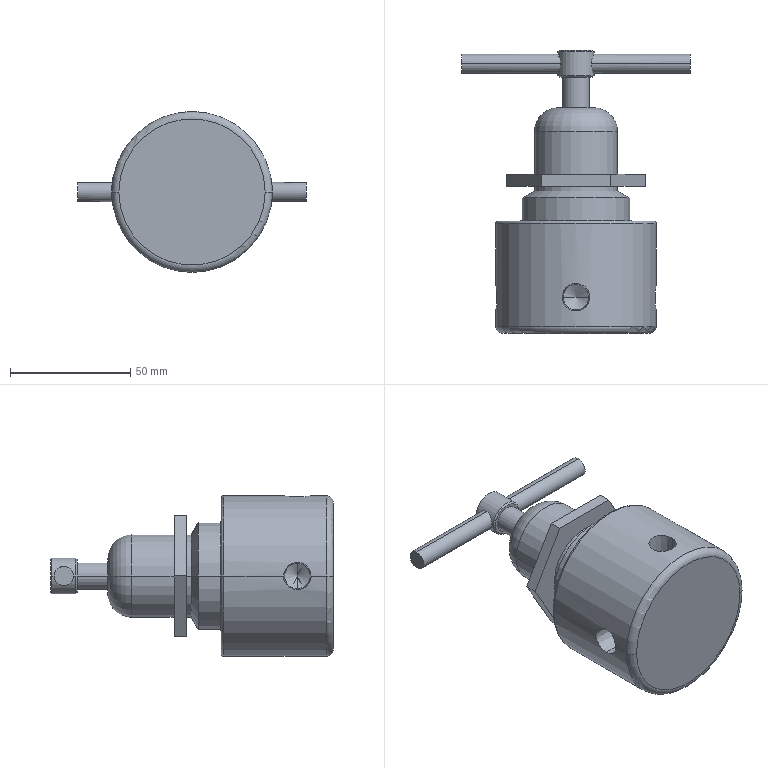Part | STEP file | 853PLX-200-N | 2 solids | 67 faces | box 95 x 117.594 x 66.785 mm | volume 220085 mm3 | cylinder 24 | plane 19 | cone 18 | torus 6 | commonest cylinder face diameters 10.7 x6 8 x4 11.227 x2 14.969 x2 34.544 x2 35 x2